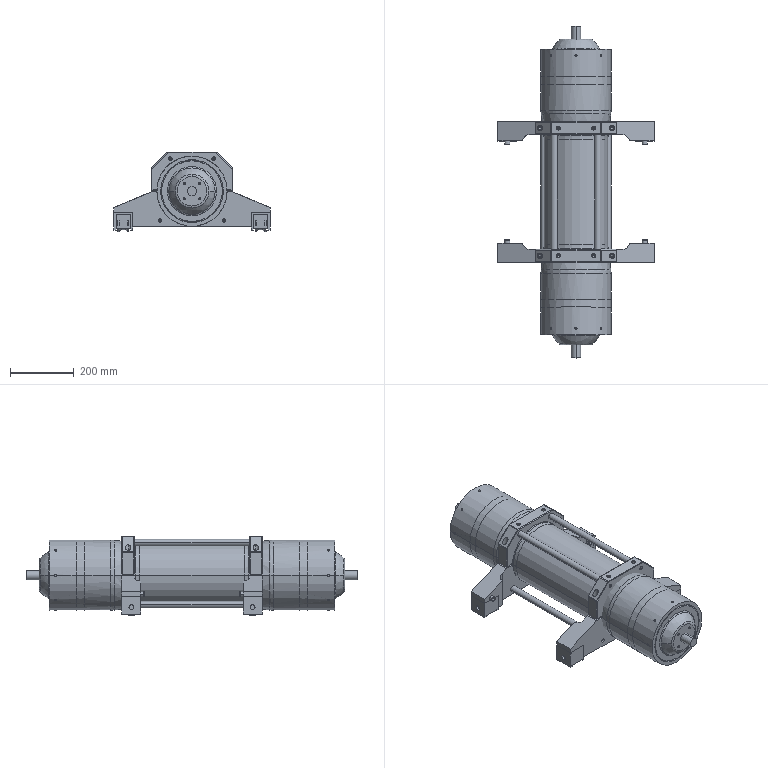Part | NX | features BREP 11 | 28 solids | 998 faces | box 490 x 1040 x 249.5 mm | volume 31359390 mm3 | cylinder 404 | plane 274 | cone 192 | torus 120 | sphere 8 | commonest cylinder face diameters 6.8 x64 8.376 x24 9.149 x24 10 x20 20 x20 4.917 x16